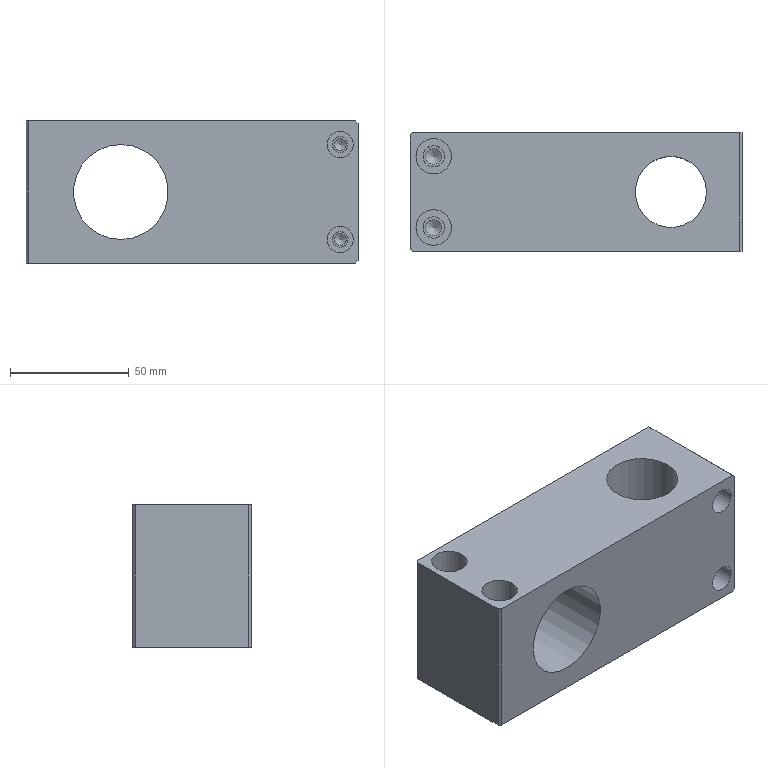Part | NX | 1 solid | 36 faces | box 140 x 50 x 60 mm | volume 301515 mm3 | plane 18 | cylinder 14 | cone 4 | commonest cylinder face diameters 5 x2 6.6 x2 6.8 x2 9 x2 11 x2 15 x2
STEP:
#1=CARTESIAN_POINT('',(62.5,1.5,7.5));
#2=VERTEX_POINT('',#1);
#3=CARTESIAN_POINT('',(62.5,1.5,10.));
#4=DIRECTION('',(0.,-1.,0.));
#5=DIRECTION('',(0.,0.,-1.));
#6=AXIS2_PLACEMENT_3D('',#3,#4,#5);
#7=CIRCLE('',#6,2.5);
#8=EDGE_CURVE('',#2,#2,#7,.T.);
#9=ORIENTED_EDGE('',*,*,#8,.F.);
#10=EDGE_LOOP('',(#9));
#11=FACE_BOUND('',#10,.T.);
#12=CARTESIAN_POINT('',(59.2,1.5,10.));
#13=VERTEX_POINT('',#12);
#14=CARTESIAN_POINT('',(62.5,1.5,10.));
#15=DIRECTION('',(0.,1.,0.));
#16=DIRECTION('',(-1.,0.,0.));
#17=AXIS2_PLACEMENT_3D('',#14,#15,#16);
#18=CIRCLE('',#17,3.3);
#19=EDGE_CURVE('',#13,#13,#18,.T.);
#20=ORIENTED_EDGE('',*,*,#19,.F.);
#21=EDGE_LOOP('',(#20));
#22=FACE_BOUND('',#21,.T.);
#23=CARTESIAN_POINT('',(20.,1.5,60.));
#24=DIRECTION('',(0.,1.,0.));
#25=DIRECTION('',(-1.,0.,0.));
#26=AXIS2_PLACEMENT_3D('',#23,#24,#25);
#27=PLANE('',#26);
#28=ADVANCED_FACE('',(#11,#22),#27,.F.);
#29=CARTESIAN_POINT('',(62.5,1.5,47.5));
#30=VERTEX_POINT('',#29);
#31=CARTESIAN_POINT('',(62.5,1.5,50.));
#32=DIRECTION('',(0.,-1.,0.));
#33=DIRECTION('',(0.,0.,-1.));
#34=AXIS2_PLACEMENT_3D('',#31,#32,#33);
#35=CIRCLE('',#34,2.5);
#36=EDGE_CURVE('',#30,#30,#35,.T.);
#37=ORIENTED_EDGE('',*,*,#36,.F.);
#38=EDGE_LOOP('',(#37));
#39=FACE_BOUND('',#38,.T.);
#40=CARTESIAN_POINT('',(59.2,1.5,50.));
#41=VERTEX_POINT('',#40);
#42=CARTESIAN_POINT('',(62.5,1.5,50.));
#43=DIRECTION('',(0.,1.,0.));
#44=DIRECTION('',(-1.,0.,0.));
#45=AXIS2_PLACEMENT_3D('',#42,#43,#44);
#46=CIRCLE('',#45,3.3);
#47=EDGE_CURVE('',#41,#41,#46,.T.);
#48=ORIENTED_EDGE('',*,*,#47,.F.);
#49=EDGE_LOOP('',(#48));
#50=FACE_BOUND('',#49,.T.);
#51=CARTESIAN_POINT('',(20.,1.5,60.));
#52=DIRECTION('',(0.,1.,0.));
#53=DIRECTION('',(-1.,0.,0.));
#54=AXIS2_PLACEMENT_3D('',#51,#52,#53);
#55=PLANE('',#54);
#56=ADVANCED_FACE('',(#39,#50),#55,.F.);
#57=CARTESIAN_POINT('',(-56.6,-15.,28.5));
#58=VERTEX_POINT('',#57);
#59=CARTESIAN_POINT('',(-60.,-15.,28.5));
#60=DIRECTION('',(0.,0.,1.));
#61=DIRECTION('',(1.,0.,0.));
#62=AXIS2_PLACEMENT_3D('',#59,#60,#61);
#63=CIRCLE('',#62,3.4);
#64=EDGE_CURVE('',#58,#58,#63,.T.);
#65=ORIENTED_EDGE('',*,*,#64,.F.);
#66=EDGE_LOOP('',(#65));
#67=FACE_BOUND('',#66,.T.);
#68=CARTESIAN_POINT('',(-64.5,-15.,28.5));
#69=VERTEX_POINT('',#68);
#70=CARTESIAN_POINT('',(-60.,-15.,28.5));
#71=DIRECTION('',(0.,0.,-1.));
#72=DIRECTION('',(-1.,0.,0.));
#73=AXIS2_PLACEMENT_3D('',#70,#71,#72);
#74=CIRCLE('',#73,4.5);
#75=EDGE_CURVE('',#69,#69,#74,.T.);
#76=ORIENTED_EDGE('',*,*,#75,.F.);
#77=EDGE_LOOP('',(#76));
#78=FACE_BOUND('',#77,.T.);
#79=CARTESIAN_POINT('',(-70.,25.,28.5));
#80=DIRECTION('',(0.,0.,-1.));
#81=DIRECTION('',(-1.,0.,0.));
#82=AXIS2_PLACEMENT_3D('',#79,#80,#81);
#83=PLANE('',#82);
#84=ADVANCED_FACE('',(#67,#78),#83,.F.);
#85=CARTESIAN_POINT('',(-56.6,15.,28.5));
#86=VERTEX_POINT('',#85);
#87=CARTESIAN_POINT('',(-60.,15.,28.5));
#88=DIRECTION('',(0.,0.,1.));
#89=DIRECTION('',(1.,0.,0.));
#90=AXIS2_PLACEMENT_3D('',#87,#88,#89);
#91=CIRCLE('',#90,3.4);
#92=EDGE_CURVE('',#86,#86,#91,.T.);
#93=ORIENTED_EDGE('',*,*,#92,.F.);
#94=EDGE_LOOP('',(#93));
#95=FACE_BOUND('',#94,.T.);
#96=CARTESIAN_POINT('',(-64.5,15.,28.5));
#97=VERTEX_POINT('',#96);
#98=CARTESIAN_POINT('',(-60.,15.,28.5));
#99=DIRECTION('',(0.,0.,-1.));
#100=DIRECTION('',(-1.,0.,0.));
#101=AXIS2_PLACEMENT_3D('',#98,#99,#100);
#102=CIRCLE('',#101,4.5);
#103=EDGE_CURVE('',#97,#97,#102,.T.);
#104=ORIENTED_EDGE('',*,*,#103,.F.);
#105=EDGE_LOOP('',(#104));
#106=FACE_BOUND('',#105,.T.);
#107=CARTESIAN_POINT('',(-70.,25.,28.5));
#108=DIRECTION('',(0.,0.,-1.));
#109=DIRECTION('',(-1.,0.,0.));
#110=AXIS2_PLACEMENT_3D('',#107,#108,#109);
#111=PLANE('',#110);
#112=ADVANCED_FACE('',(#95,#106),#111,.F.);
#113=CARTESIAN_POINT('',(-70.,24.,0.));
#114=VERTEX_POINT('',#113);
#115=CARTESIAN_POINT('',(-69.,25.,0.));
#116=VERTEX_POINT('',#115);
#117=CARTESIAN_POINT('',(-47.,47.,0.));
#118=DIRECTION('',(0.7071,0.7071,0.));
#119=VECTOR('',#118,1000.);
#120=LINE('',#117,#119);
#121=EDGE_CURVE('',#114,#116,#120,.T.);
#122=ORIENTED_EDGE('',*,*,#121,.F.);
#123=CARTESIAN_POINT('',(-70.,24.,60.));
#124=VERTEX_POINT('',#123);
#125=CARTESIAN_POINT('',(-70.,24.,60.));
#126=DIRECTION('',(0.,0.,-1.));
#127=VECTOR('',#126,1000.);
#128=LINE('',#125,#127);
#129=EDGE_CURVE('',#124,#114,#128,.T.);
#130=ORIENTED_EDGE('',*,*,#129,.F.);
#131=CARTESIAN_POINT('',(-69.,25.,60.));
#132=VERTEX_POINT('',#131);
#133=CARTESIAN_POINT('',(-70.,24.,60.));
#134=DIRECTION('',(-0.7071,-0.7071,0.));
#135=VECTOR('',#134,1000.);
#136=LINE('',#133,#135);
#137=EDGE_CURVE('',#132,#124,#136,.T.);
#138=ORIENTED_EDGE('',*,*,#137,.F.);
#139=CARTESIAN_POINT('',(-69.,25.,60.));
#140=DIRECTION('',(0.,0.,1.));
#141=VECTOR('',#140,1000.);
#142=LINE('',#139,#141);
#143=EDGE_CURVE('',#116,#132,#142,.T.);
#144=ORIENTED_EDGE('',*,*,#143,.F.);
#145=EDGE_LOOP('',(#122,#130,#138,#144));
#146=FACE_BOUND('',#145,.T.);
#147=CARTESIAN_POINT('',(-70.,24.,60.));
#148=DIRECTION('',(0.7071,-0.7071,0.));
#149=DIRECTION('',(0.,0.,-1.));
#150=AXIS2_PLACEMENT_3D('',#147,#148,#149);
#151=PLANE('',#150);
#152=ADVANCED_FACE('',(#146),#151,.F.);
#153=CARTESIAN_POINT('',(-69.,-25.,0.));
#154=VERTEX_POINT('',#153);
#155=CARTESIAN_POINT('',(-70.,-24.,0.));
#156=VERTEX_POINT('',#155);
#157=CARTESIAN_POINT('',(-47.,-47.,0.));
#158=DIRECTION('',(-0.7071,0.7071,0.));
#159=VECTOR('',#158,1000.);
#160=LINE('',#157,#159);
#161=EDGE_CURVE('',#154,#156,#160,.T.);
#162=ORIENTED_EDGE('',*,*,#161,.F.);
#163=CARTESIAN_POINT('',(-69.,-25.,60.));
#164=VERTEX_POINT('',#163);
#165=CARTESIAN_POINT('',(-69.,-25.,60.));
#166=DIRECTION('',(0.,0.,-1.));
#167=VECTOR('',#166,1000.);
#168=LINE('',#165,#167);
#169=EDGE_CURVE('',#164,#154,#168,.T.);
#170=ORIENTED_EDGE('',*,*,#169,.F.);
#171=CARTESIAN_POINT('',(-70.,-24.,60.));
#172=VERTEX_POINT('',#171);
#173=CARTESIAN_POINT('',(-69.,-25.,60.));
#174=DIRECTION('',(0.7071,-0.7071,0.));
#175=VECTOR('',#174,1000.);
#176=LINE('',#173,#175);
#177=EDGE_CURVE('',#172,#164,#176,.T.);
#178=ORIENTED_EDGE('',*,*,#177,.F.);
#179=CARTESIAN_POINT('',(-70.,-24.,60.));
#180=DIRECTION('',(0.,0.,1.));
#181=VECTOR('',#180,1000.);
#182=LINE('',#179,#181);
#183=EDGE_CURVE('',#156,#172,#182,.T.);
#184=ORIENTED_EDGE('',*,*,#183,.F.);
#185=EDGE_LOOP('',(#162,#170,#178,#184));
#186=FACE_BOUND('',#185,.T.);
#187=CARTESIAN_POINT('',(-69.,-25.,60.));
#188=DIRECTION('',(0.7071,0.7071,0.));
#189=DIRECTION('',(0.,0.,-1.));
#190=AXIS2_PLACEMENT_3D('',#187,#188,#189);
#191=PLANE('',#190);
#192=ADVANCED_FACE('',(#186),#191,.F.);
#193=CARTESIAN_POINT('',(69.,-25.,60.));
#194=VERTEX_POINT('',#193);
#195=CARTESIAN_POINT('',(69.,25.,60.));
#196=VERTEX_POINT('',#195);
#197=CARTESIAN_POINT('',(69.,0.,60.));
#198=DIRECTION('',(0.,1.,0.));
#199=VECTOR('',#198,1000.);
#200=LINE('',#197,#199);
#201=EDGE_CURVE('',#194,#196,#200,.T.);
#202=ORIENTED_EDGE('',*,*,#201,.F.);
#203=CARTESIAN_POINT('',(70.,-25.,59.));
#204=VERTEX_POINT('',#203);
#205=CARTESIAN_POINT('',(69.,-25.,60.));
#206=DIRECTION('',(-0.7071,0.,0.7071));
#207=VECTOR('',#206,1000.);
#208=LINE('',#205,#207);
#209=EDGE_CURVE('',#204,#194,#208,.T.);
#210=ORIENTED_EDGE('',*,*,#209,.F.);
#211=CARTESIAN_POINT('',(70.,25.,59.));
#212=VERTEX_POINT('',#211);
#213=CARTESIAN_POINT('',(70.,-25.,59.));
#214=DIRECTION('',(0.,-1.,0.));
#215=VECTOR('',#214,1000.);
#216=LINE('',#213,#215);
#217=EDGE_CURVE('',#212,#204,#216,.T.);
#218=ORIENTED_EDGE('',*,*,#217,.F.);
#219=CARTESIAN_POINT('',(69.,25.,60.));
#220=DIRECTION('',(0.7071,0.,-0.7071));
#221=VECTOR('',#220,1000.);
#222=LINE('',#219,#221);
#223=EDGE_CURVE('',#196,#212,#222,.T.);
#224=ORIENTED_EDGE('',*,*,#223,.F.);
#225=EDGE_LOOP('',(#202,#210,#218,#224));
#226=FACE_BOUND('',#225,.T.);
#227=CARTESIAN_POINT('',(69.,0.,60.));
#228=DIRECTION('',(-0.7071,0.,-0.7071));
#229=DIRECTION('',(0.,1.,0.));
#230=AXIS2_PLACEMENT_3D('',#227,#228,#229);
#231=PLANE('',#230);
#232=ADVANCED_FACE('',(#226),#231,.F.);
#233=CARTESIAN_POINT('',(69.,-25.,0.));
#234=VERTEX_POINT('',#233);
#235=CARTESIAN_POINT('',(70.,-25.,1.));
#236=VERTEX_POINT('',#235);
#237=CARTESIAN_POINT('',(70.,-25.,1.));
#238=DIRECTION('',(0.7071,0.,0.7071));
#239=VECTOR('',#238,1000.);
#240=LINE('',#237,#239);
#241=EDGE_CURVE('',#234,#236,#240,.T.);
#242=ORIENTED_EDGE('',*,*,#241,.F.);
#243=CARTESIAN_POINT('',(69.,25.,0.));
#244=VERTEX_POINT('',#243);
#245=CARTESIAN_POINT('',(69.,-25.,0.));
#246=DIRECTION('',(0.,-1.,0.));
#247=VECTOR('',#246,1000.);
#248=LINE('',#245,#247);
#249=EDGE_CURVE('',#244,#234,#248,.T.);
#250=ORIENTED_EDGE('',*,*,#249,.F.);
#251=CARTESIAN_POINT('',(70.,25.,1.));
#252=VERTEX_POINT('',#251);
#253=CARTESIAN_POINT('',(70.,25.,1.));
#254=DIRECTION('',(-0.7071,0.,-0.7071));
#255=VECTOR('',#254,1000.);
#256=LINE('',#253,#255);
#257=EDGE_CURVE('',#252,#244,#256,.T.);
#258=ORIENTED_EDGE('',*,*,#257,.F.);
#259=CARTESIAN_POINT('',(70.,-1.5,1.));
#260=DIRECTION('',(0.,1.,0.));
#261=VECTOR('',#260,1000.);
#262=LINE('',#259,#261);
#263=EDGE_CURVE('',#236,#252,#262,.T.);
#264=ORIENTED_EDGE('',*,*,#263,.F.);
#265=EDGE_LOOP('',(#242,#250,#258,#264));
#266=FACE_BOUND('',#265,.T.);
#267=CARTESIAN_POINT('',(70.,-25.,1.));
#268=DIRECTION('',(0.7071,0.,-0.7071));
#269=DIRECTION('',(0.,-1.,0.));
#270=AXIS2_PLACEMENT_3D('',#267,#268,#269);
#271=PLANE('',#270);
#272=ADVANCED_FACE('',(#266),#271,.T.);
#273=CARTESIAN_POINT('',(-52.5,15.,45.));
#274=VERTEX_POINT('',#273);
#275=CARTESIAN_POINT('',(-60.,15.,45.));
#276=DIRECTION('',(0.,0.,1.));
#277=DIRECTION('',(1.,0.,0.));
#278=AXIS2_PLACEMENT_3D('',#275,#276,#277);
#279=CIRCLE('',#278,7.5);
#280=EDGE_CURVE('',#274,#274,#279,.T.);
#281=ORIENTED_EDGE('',*,*,#280,.T.);
#282=EDGE_LOOP('',(#281));
#283=FACE_BOUND('',#282,.T.);
#284=CARTESIAN_POINT('',(-55.5,15.,45.));
#285=VERTEX_POINT('',#284);
#286=CARTESIAN_POINT('',(-60.,15.,45.));
#287=DIRECTION('',(0.,0.,1.));
#288=DIRECTION('',(1.,0.,0.));
#289=AXIS2_PLACEMENT_3D('',#286,#287,#288);
#290=CIRCLE('',#289,4.5);
#291=EDGE_CURVE('',#285,#285,#290,.T.);
#292=ORIENTED_EDGE('',*,*,#291,.F.);
#293=EDGE_LOOP('',(#292));
#294=FACE_BOUND('',#293,.T.);
#295=CARTESIAN_POINT('',(-55.5,15.,45.));
#296=DIRECTION('',(0.,0.,-1.));
#297=DIRECTION('',(-1.,0.,0.));
#298=AXIS2_PLACEMENT_3D('',#295,#296,#297);
#299=PLANE('',#298);
#300=ADVANCED_FACE('',(#283,#294),#299,.F.);
#301=CARTESIAN_POINT('',(-67.5,-15.,45.));
#302=VERTEX_POINT('',#301);
#303=CARTESIAN_POINT('',(-60.,-15.,45.));
#304=DIRECTION('',(0.,0.,1.));
#305=DIRECTION('',(-1.,0.,0.));
#306=AXIS2_PLACEMENT_3D('',#303,#304,#305);
#307=CIRCLE('',#306,7.5);
#308=EDGE_CURVE('',#302,#302,#307,.T.);
#309=ORIENTED_EDGE('',*,*,#308,.T.);
#310=EDGE_LOOP('',(#309));
#311=FACE_BOUND('',#310,.T.);
#312=CARTESIAN_POINT('',(-64.5,-15.,45.));
#313=VERTEX_POINT('',#312);
#314=CARTESIAN_POINT('',(-60.,-15.,45.));
#315=DIRECTION('',(0.,0.,1.));
#316=DIRECTION('',(-1.,0.,0.));
#317=AXIS2_PLACEMENT_3D('',#314,#315,#316);
#318=CIRCLE('',#317,4.5);
#319=EDGE_CURVE('',#313,#313,#318,.T.);
#320=ORIENTED_EDGE('',*,*,#319,.F.);
#321=EDGE_LOOP('',(#320));
#322=FACE_BOUND('',#321,.T.);
#323=CARTESIAN_POINT('',(-55.5,15.,45.));
#324=DIRECTION('',(0.,0.,-1.));
#325=DIRECTION('',(-1.,0.,0.));
#326=AXIS2_PLACEMENT_3D('',#323,#324,#325);
#327=PLANE('',#326);
#328=ADVANCED_FACE('',(#311,#322),#327,.F.);
#329=CARTESIAN_POINT('',(62.5,-10.,44.5));
#330=VERTEX_POINT('',#329);
#331=CARTESIAN_POINT('',(62.5,-10.,50.));
#332=DIRECTION('',(0.,-1.,0.));
#333=DIRECTION('',(0.,0.,-1.));
#334=AXIS2_PLACEMENT_3D('',#331,#332,#333);
#335=CIRCLE('',#334,5.5);
#336=EDGE_CURVE('',#330,#330,#335,.T.);
#337=ORIENTED_EDGE('',*,*,#336,.T.);
#338=EDGE_LOOP('',(#337));
#339=FACE_BOUND('',#338,.T.);
#340=CARTESIAN_POINT('',(62.5,-10.,46.7));
#341=VERTEX_POINT('',#340);
#342=CARTESIAN_POINT('',(62.5,-10.,50.));
#343=DIRECTION('',(0.,-1.,0.));
#344=DIRECTION('',(0.,0.,-1.));
#345=AXIS2_PLACEMENT_3D('',#342,#343,#344);
#346=CIRCLE('',#345,3.3);
#347=EDGE_CURVE('',#341,#341,#346,.T.);
#348=ORIENTED_EDGE('',*,*,#347,.F.);
#349=EDGE_LOOP('',(#348));
#350=FACE_BOUND('',#349,.T.);
#351=CARTESIAN_POINT('',(65.8,-10.,50.));
#352=DIRECTION('',(0.,1.,0.));
#353=DIRECTION('',(0.,0.,1.));
#354=AXIS2_PLACEMENT_3D('',#351,#352,#353);
#355=PLANE('',#354);
#356=ADVANCED_FACE('',(#339,#350),#355,.F.);
#357=CARTESIAN_POINT('',(62.5,-10.,15.5));
#358=VERTEX_POINT('',#357);
#359=CARTESIAN_POINT('',(62.5,-10.,10.));
#360=DIRECTION('',(0.,-1.,0.));
#361=DIRECTION('',(0.,0.,1.));
#362=AXIS2_PLACEMENT_3D('',#359,#360,#361);
#363=CIRCLE('',#362,5.5);
#364=EDGE_CURVE('',#358,#358,#363,.T.);
#365=ORIENTED_EDGE('',*,*,#364,.T.);
#366=EDGE_LOOP('',(#365));
#367=FACE_BOUND('',#366,.T.);
#368=CARTESIAN_POINT('',(62.5,-10.,13.3));
#369=VERTEX_POINT('',#368);
#370=CARTESIAN_POINT('',(62.5,-10.,10.));
#371=DIRECTION('',(0.,-1.,0.));
#372=DIRECTION('',(0.,0.,1.));
#373=AXIS2_PLACEMENT_3D('',#370,#371,#372);
#374=CIRCLE('',#373,3.3);
#375=EDGE_CURVE('',#369,#369,#374,.T.);
#376=ORIENTED_EDGE('',*,*,#375,.F.);
#377=EDGE_LOOP('',(#376));
#378=FACE_BOUND('',#377,.T.);
#379=CARTESIAN_POINT('',(65.8,-10.,50.));
#380=DIRECTION('',(0.,1.,0.));
#381=DIRECTION('',(0.,0.,1.));
#382=AXIS2_PLACEMENT_3D('',#379,#380,#381);
#383=PLANE('',#382);
#384=ADVANCED_FACE('',(#367,#378),#383,.F.);
#385=CARTESIAN_POINT('',(-70.,25.,0.));
#386=DIRECTION('',(-1.,0.,0.));
#387=VECTOR('',#386,1000.);
#388=LINE('',#385,#387);
#389=EDGE_CURVE('',#244,#116,#388,.T.);
#390=ORIENTED_EDGE('',*,*,#389,.F.);
#391=ORIENTED_EDGE('',*,*,#249,.T.);
#392=CARTESIAN_POINT('',(-70.,-25.,0.));
#393=DIRECTION('',(1.,0.,0.));
#394=VECTOR('',#393,1000.);
#395=LINE('',#392,#394);
#396=EDGE_CURVE('',#154,#234,#395,.T.);
#397=ORIENTED_EDGE('',*,*,#396,.F.);
#398=ORIENTED_EDGE('',*,*,#161,.T.);
#399=CARTESIAN_POINT('',(-70.,-25.,0.));
#400=DIRECTION('',(0.,-1.,0.));
#401=VECTOR('',#400,1000.);
#402=LINE('',#399,#401);
#403=EDGE_CURVE('',#114,#156,#402,.T.);
#404=ORIENTED_EDGE('',*,*,#403,.F.);
#405=ORIENTED_EDGE('',*,*,#121,.T.);
#406=EDGE_LOOP('',(#390,#391,#397,#398,#404,#405));
#407=FACE_BOUND('',#406,.T.);
#408=CARTESIAN_POINT('',(55.,0.,0.));
#409=VERTEX_POINT('',#408);
#410=CARTESIAN_POINT('',(40.,0.,0.));
#411=DIRECTION('',(0.,0.,1.));
#412=DIRECTION('',(1.,0.,0.));
#413=AXIS2_PLACEMENT_3D('',#410,#411,#412);
#414=CIRCLE('',#413,15.);
#415=EDGE_CURVE('',#409,#409,#414,.T.);
#416=ORIENTED_EDGE('',*,*,#415,.T.);
#417=EDGE_LOOP('',(#416));
#418=FACE_BOUND('',#417,.T.);
#419=CARTESIAN_POINT('',(0.,0.,0.));
#420=DIRECTION('',(0.,0.,-1.));
#421=DIRECTION('',(-1.,0.,0.));
#422=AXIS2_PLACEMENT_3D('',#419,#420,#421);
#423=PLANE('',#422);
#424=ADVANCED_FACE('',(#407,#418),#423,.T.);
#425=CARTESIAN_POINT('',(-30.,-25.,50.));
#426=VERTEX_POINT('',#425);
#427=CARTESIAN_POINT('',(-30.,-25.,30.));
#428=DIRECTION('',(0.,1.,0.));
#429=DIRECTION('',(0.,0.,1.));
#430=AXIS2_PLACEMENT_3D('',#427,#428,#429);
#431=CIRCLE('',#430,20.);
#432=EDGE_CURVE('',#426,#426,#431,.T.);
#433=ORIENTED_EDGE('',*,*,#432,.T.);
#434=EDGE_LOOP('',(#433));
#435=FACE_BOUND('',#434,.T.);
#436=ORIENTED_EDGE('',*,*,#396,.T.);
#437=ORIENTED_EDGE('',*,*,#241,.T.);
#438=CARTESIAN_POINT('',(70.,-25.,60.));
#439=DIRECTION('',(0.,0.,-1.));
#440=VECTOR('',#439,1000.);
#441=LINE('',#438,#440);
#442=EDGE_CURVE('',#204,#236,#441,.T.);
#443=ORIENTED_EDGE('',*,*,#442,.F.);
#444=ORIENTED_EDGE('',*,*,#209,.T.);
#445=CARTESIAN_POINT('',(-70.,-25.,60.));
#446=DIRECTION('',(1.,0.,0.));
#447=VECTOR('',#446,1000.);
#448=LINE('',#445,#447);
#449=EDGE_CURVE('',#164,#194,#448,.T.);
#450=ORIENTED_EDGE('',*,*,#449,.F.);
#451=ORIENTED_EDGE('',*,*,#169,.T.);
#452=EDGE_LOOP('',(#436,#437,#443,#444,#450,#451));
#453=FACE_BOUND('',#452,.T.);
#454=CARTESIAN_POINT('',(62.5,-25.,4.5));
#455=VERTEX_POINT('',#454);
#456=CARTESIAN_POINT('',(62.5,-25.,10.));
#457=DIRECTION('',(0.,-1.,0.));
#458=DIRECTION('',(0.,0.,-1.));
#459=AXIS2_PLACEMENT_3D('',#456,#457,#458);
#460=CIRCLE('',#459,5.5);
#461=EDGE_CURVE('',#455,#455,#460,.T.);
#462=ORIENTED_EDGE('',*,*,#461,.F.);
#463=EDGE_LOOP('',(#462));
#464=FACE_BOUND('',#463,.T.);
#465=CARTESIAN_POINT('',(62.5,-25.,44.5));
#466=VERTEX_POINT('',#465);
#467=CARTESIAN_POINT('',(62.5,-25.,50.));
#468=DIRECTION('',(0.,-1.,0.));
#469=DIRECTION('',(0.,0.,-1.));
#470=AXIS2_PLACEMENT_3D('',#467,#468,#469);
#471=CIRCLE('',#470,5.5);
#472=EDGE_CURVE('',#466,#466,#471,.T.);
#473=ORIENTED_EDGE('',*,*,#472,.F.);
#474=EDGE_LOOP('',(#473));
#475=FACE_BOUND('',#474,.T.);
#476=CARTESIAN_POINT('',(-70.,-25.,60.));
#477=DIRECTION('',(0.,1.,0.));
#478=DIRECTION('',(0.,0.,1.));
#479=AXIS2_PLACEMENT_3D('',#476,#477,#478);
#480=PLANE('',#479);
#481=ADVANCED_FACE('',(#435,#453,#464,#475),#480,.F.);
#482=CARTESIAN_POINT('',(-30.,25.,50.));
#483=VERTEX_POINT('',#482);
#484=CARTESIAN_POINT('',(-30.,25.,30.));
#485=DIRECTION('',(0.,1.,0.));
#486=DIRECTION('',(0.,0.,1.));
#487=AXIS2_PLACEMENT_3D('',#484,#485,#486);
#488=CIRCLE('',#487,20.);
#489=EDGE_CURVE('',#483,#483,#488,.T.);
#490=ORIENTED_EDGE('',*,*,#489,.F.);
#491=EDGE_LOOP('',(#490));
#492=FACE_BOUND('',#491,.T.);
#493=CARTESIAN_POINT('',(70.,25.,60.));
#494=DIRECTION('',(0.,0.,-1.));
#495=VECTOR('',#494,1000.);
#496=LINE('',#493,#495);
#497=EDGE_CURVE('',#212,#252,#496,.T.);
#498=ORIENTED_EDGE('',*,*,#497,.T.);
#499=ORIENTED_EDGE('',*,*,#257,.T.);
#500=ORIENTED_EDGE('',*,*,#389,.T.);
#501=ORIENTED_EDGE('',*,*,#143,.T.);
#502=CARTESIAN_POINT('',(-70.,25.,60.));
#503=DIRECTION('',(-1.,0.,0.));
#504=VECTOR('',#503,1000.);
#505=LINE('',#502,#504);
#506=EDGE_CURVE('',#196,#132,#505,.T.);
#507=ORIENTED_EDGE('',*,*,#506,.F.);
#508=ORIENTED_EDGE('',*,*,#223,.T.);
#509=EDGE_LOOP('',(#498,#499,#500,#501,#507,#508));
#510=FACE_BOUND('',#509,.T.);
#511=CARTESIAN_POINT('',(-70.,25.,60.));
#512=DIRECTION('',(0.,-1.,0.));
#513=DIRECTION('',(0.,0.,-1.));
#514=AXIS2_PLACEMENT_3D('',#511,#512,#513);
#515=PLANE('',#514);
#516=ADVANCED_FACE('',(#492,#510),#515,.F.);
#517=CARTESIAN_POINT('',(-70.,-25.,60.));
#518=DIRECTION('',(0.,-1.,0.));
#519=VECTOR('',#518,1000.);
#520=LINE('',#517,#519);
#521=EDGE_CURVE('',#124,#172,#520,.T.);
#522=ORIENTED_EDGE('',*,*,#521,.F.);
#523=ORIENTED_EDGE('',*,*,#129,.T.);
#524=ORIENTED_EDGE('',*,*,#403,.T.);
#525=ORIENTED_EDGE('',*,*,#183,.T.);
#526=EDGE_LOOP('',(#522,#523,#524,#525));
#527=FACE_BOUND('',#526,.T.);
#528=CARTESIAN_POINT('',(-70.,-25.,60.));
#529=DIRECTION('',(1.,0.,0.));
#530=DIRECTION('',(0.,0.,-1.));
#531=AXIS2_PLACEMENT_3D('',#528,#529,#530);
#532=PLANE('',#531);
#533=ADVANCED_FACE('',(#527),#532,.F.);
#534=ORIENTED_EDGE('',*,*,#415,.F.);
#535=EDGE_LOOP('',(#534));
#536=FACE_BOUND('',#535,.T.);
#537=CARTESIAN_POINT('',(55.,0.,60.));
#538=VERTEX_POINT('',#537);
#539=CARTESIAN_POINT('',(40.,0.,60.));
#540=DIRECTION('',(0.,0.,1.));
#541=DIRECTION('',(1.,0.,0.));
#542=AXIS2_PLACEMENT_3D('',#539,#540,#541);
#543=CIRCLE('',#542,15.);
#544=EDGE_CURVE('',#538,#538,#543,.T.);
#545=ORIENTED_EDGE('',*,*,#544,.T.);
#546=EDGE_LOOP('',(#545));
#547=FACE_BOUND('',#546,.T.);
#548=CARTESIAN_POINT('',(40.,0.,0.));
#549=DIRECTION('',(0.,0.,1.));
#550=DIRECTION('',(1.,0.,0.));
#551=AXIS2_PLACEMENT_3D('',#548,#549,#550);
#552=CYLINDRICAL_SURFACE('',#551,15.);
#553=ADVANCED_FACE('',(#536,#547),#552,.F.);
#554=ORIENTED_EDGE('',*,*,#442,.T.);
#555=ORIENTED_EDGE('',*,*,#263,.T.);
#556=ORIENTED_EDGE('',*,*,#497,.F.);
#557=ORIENTED_EDGE('',*,*,#217,.T.);
#558=EDGE_LOOP('',(#554,#555,#556,#557));
#559=FACE_BOUND('',#558,.T.);
#560=CARTESIAN_POINT('',(70.,-25.,60.));
#561=DIRECTION('',(-1.,0.,0.));
#562=DIRECTION('',(0.,0.,1.));
#563=AXIS2_PLACEMENT_3D('',#560,#561,#562);
#564=PLANE('',#563);
#565=ADVANCED_FACE('',(#559),#564,.F.);
#566=ORIENTED_EDGE('',*,*,#449,.T.);
#567=ORIENTED_EDGE('',*,*,#201,.T.);
#568=ORIENTED_EDGE('',*,*,#506,.T.);
#569=ORIENTED_EDGE('',*,*,#137,.T.);
#570=ORIENTED_EDGE('',*,*,#521,.T.);
#571=ORIENTED_EDGE('',*,*,#177,.T.);
#572=EDGE_LOOP('',(#566,#567,#568,#569,#570,#571));
#573=FACE_BOUND('',#572,.T.);
#574=CARTESIAN_POINT('',(-52.5,15.,60.));
#575=VERTEX_POINT('',#574);
#576=CARTESIAN_POINT('',(-60.,15.,60.));
#577=DIRECTION('',(0.,0.,1.));
#578=DIRECTION('',(1.,0.,0.));
#579=AXIS2_PLACEMENT_3D('',#576,#577,#578);
#580=CIRCLE('',#579,7.5);
#581=EDGE_CURVE('',#575,#575,#580,.T.);
#582=ORIENTED_EDGE('',*,*,#581,.F.);
#583=EDGE_LOOP('',(#582));
#584=FACE_BOUND('',#583,.T.);
#585=ORIENTED_EDGE('',*,*,#544,.F.);
#586=EDGE_LOOP('',(#585));
#587=FACE_BOUND('',#586,.T.);
#588=CARTESIAN_POINT('',(-52.5,-15.,60.));
#589=VERTEX_POINT('',#588);
#590=CARTESIAN_POINT('',(-60.,-15.,60.));
#591=DIRECTION('',(0.,0.,1.));
#592=DIRECTION('',(1.,0.,0.));
#593=AXIS2_PLACEMENT_3D('',#590,#591,#592);
#594=CIRCLE('',#593,7.5);
#595=EDGE_CURVE('',#589,#589,#594,.T.);
#596=ORIENTED_EDGE('',*,*,#595,.F.);
#597=EDGE_LOOP('',(#596));
#598=FACE_BOUND('',#597,.T.);
#599=CARTESIAN_POINT('',(0.,0.,60.));
#600=DIRECTION('',(0.,0.,-1.));
#601=DIRECTION('',(-1.,0.,0.));
#602=AXIS2_PLACEMENT_3D('',#599,#600,#601);
#603=PLANE('',#602);
#604=ADVANCED_FACE('',(#573,#584,#587,#598),#603,.F.);
#605=ORIENTED_EDGE('',*,*,#489,.T.);
#606=EDGE_LOOP('',(#605));
#607=FACE_BOUND('',#606,.T.);
#608=ORIENTED_EDGE('',*,*,#432,.F.);
#609=EDGE_LOOP('',(#608));
#610=FACE_BOUND('',#609,.T.);
#611=CARTESIAN_POINT('',(-30.,-25.,30.));
#612=DIRECTION('',(0.,1.,0.));
#613=DIRECTION('',(0.,0.,1.));
#614=AXIS2_PLACEMENT_3D('',#611,#612,#613);
#615=CYLINDRICAL_SURFACE('',#614,20.);
#616=ADVANCED_FACE('',(#607,#610),#615,.F.);
#617=ORIENTED_EDGE('',*,*,#375,.T.);
#618=EDGE_LOOP('',(#617));
#619=FACE_BOUND('',#618,.T.);
#620=ORIENTED_EDGE('',*,*,#19,.T.);
#621=EDGE_LOOP('',(#620));
#622=FACE_BOUND('',#621,.T.);
#623=CARTESIAN_POINT('',(62.5,-25.,10.));
#624=DIRECTION('',(0.,-1.,0.));
#625=DIRECTION('',(0.,0.,-1.));
#626=AXIS2_PLACEMENT_3D('',#623,#624,#625);
#627=CYLINDRICAL_SURFACE('',#626,3.3);
#628=ADVANCED_FACE('',(#619,#622),#627,.F.);
#629=ORIENTED_EDGE('',*,*,#461,.T.);
#630=EDGE_LOOP('',(#629));
#631=FACE_BOUND('',#630,.T.);
#632=ORIENTED_EDGE('',*,*,#364,.F.);
#633=EDGE_LOOP('',(#632));
#634=FACE_BOUND('',#633,.T.);
#635=CARTESIAN_POINT('',(62.5,-25.,10.));
#636=DIRECTION('',(0.,-1.,0.));
#637=DIRECTION('',(0.,0.,-1.));
#638=AXIS2_PLACEMENT_3D('',#635,#636,#637);
#639=CYLINDRICAL_SURFACE('',#638,5.5);
#640=ADVANCED_FACE('',(#631,#634),#639,.F.);
#641=ORIENTED_EDGE('',*,*,#347,.T.);
#642=EDGE_LOOP('',(#641));
#643=FACE_BOUND('',#642,.T.);
#644=ORIENTED_EDGE('',*,*,#47,.T.);
#645=EDGE_LOOP('',(#644));
#646=FACE_BOUND('',#645,.T.);
#647=CARTESIAN_POINT('',(62.5,-25.,50.));
#648=DIRECTION('',(0.,-1.,0.));
#649=DIRECTION('',(0.,0.,-1.));
#650=AXIS2_PLACEMENT_3D('',#647,#648,#649);
#651=CYLINDRICAL_SURFACE('',#650,3.3);
#652=ADVANCED_FACE('',(#643,#646),#651,.F.);
#653=ORIENTED_EDGE('',*,*,#472,.T.);
#654=EDGE_LOOP('',(#653));
#655=FACE_BOUND('',#654,.T.);
#656=ORIENTED_EDGE('',*,*,#336,.F.);
#657=EDGE_LOOP('',(#656));
#658=FACE_BOUND('',#657,.T.);
#659=CARTESIAN_POINT('',(62.5,-25.,50.));
#660=DIRECTION('',(0.,-1.,0.));
#661=DIRECTION('',(0.,0.,-1.));
#662=AXIS2_PLACEMENT_3D('',#659,#660,#661);
#663=CYLINDRICAL_SURFACE('',#662,5.5);
#664=ADVANCED_FACE('',(#655,#658),#663,.F.);
#665=ORIENTED_EDGE('',*,*,#75,.T.);
#666=EDGE_LOOP('',(#665));
#667=FACE_BOUND('',#666,.T.);
#668=ORIENTED_EDGE('',*,*,#319,.T.);
#669=EDGE_LOOP('',(#668));
#670=FACE_BOUND('',#669,.T.);
#671=CARTESIAN_POINT('',(-60.,-15.,60.));
#672=DIRECTION('',(0.,0.,1.));
#673=DIRECTION('',(1.,0.,0.));
#674=AXIS2_PLACEMENT_3D('',#671,#672,#673);
#675=CYLINDRICAL_SURFACE('',#674,4.5);
#676=ADVANCED_FACE('',(#667,#670),#675,.F.);
#677=ORIENTED_EDGE('',*,*,#308,.F.);
#678=EDGE_LOOP('',(#677));
#679=FACE_BOUND('',#678,.T.);
#680=ORIENTED_EDGE('',*,*,#595,.T.);
#681=EDGE_LOOP('',(#680));
#682=FACE_BOUND('',#681,.T.);
#683=CARTESIAN_POINT('',(-60.,-15.,60.));
#684=DIRECTION('',(0.,0.,1.));
#685=DIRECTION('',(1.,0.,0.));
#686=AXIS2_PLACEMENT_3D('',#683,#684,#685);
#687=CYLINDRICAL_SURFACE('',#686,7.5);
#688=ADVANCED_FACE('',(#679,#682),#687,.F.);
#689=ORIENTED_EDGE('',*,*,#103,.T.);
#690=EDGE_LOOP('',(#689));
#691=FACE_BOUND('',#690,.T.);
#692=ORIENTED_EDGE('',*,*,#291,.T.);
#693=EDGE_LOOP('',(#692));
#694=FACE_BOUND('',#693,.T.);
#695=CARTESIAN_POINT('',(-60.,15.,60.));
#696=DIRECTION('',(0.,0.,1.));
#697=DIRECTION('',(1.,0.,0.));
#698=AXIS2_PLACEMENT_3D('',#695,#696,#697);
#699=CYLINDRICAL_SURFACE('',#698,4.5);
#700=ADVANCED_FACE('',(#691,#694),#699,.F.);
#701=ORIENTED_EDGE('',*,*,#280,.F.);
#702=EDGE_LOOP('',(#701));
#703=FACE_BOUND('',#702,.T.);
#704=ORIENTED_EDGE('',*,*,#581,.T.);
#705=EDGE_LOOP('',(#704));
#706=FACE_BOUND('',#705,.T.);
#707=CARTESIAN_POINT('',(-60.,15.,60.));
#708=DIRECTION('',(0.,0.,1.));
#709=DIRECTION('',(1.,0.,0.));
#710=AXIS2_PLACEMENT_3D('',#707,#708,#709);
#711=CYLINDRICAL_SURFACE('',#710,7.5);
#712=ADVANCED_FACE('',(#703,#706),#711,.F.);
#713=CARTESIAN_POINT('',(62.5,18.002,10.));
#714=VERTEX_POINT('',#713);
#715=VERTEX_LOOP('',#714);
#716=FACE_BOUND('',#715,.T.);
#717=CARTESIAN_POINT('',(62.5,16.5,7.5));
#718=VERTEX_POINT('',#717);
#719=CARTESIAN_POINT('',(62.5,16.5,10.));
#720=DIRECTION('',(0.,-1.,0.));
#721=DIRECTION('',(0.,0.,-1.));
#722=AXIS2_PLACEMENT_3D('',#719,#720,#721);
#723=CIRCLE('',#722,2.5);
#724=EDGE_CURVE('',#718,#718,#723,.T.);
#725=ORIENTED_EDGE('',*,*,#724,.T.);
#726=EDGE_LOOP('',(#725));
#727=FACE_BOUND('',#726,.T.);
#728=CARTESIAN_POINT('',(62.5,16.5,10.));
#729=DIRECTION('',(0.,-1.,0.));
#730=DIRECTION('',(0.,0.,-1.));
#731=AXIS2_PLACEMENT_3D('',#728,#729,#730);
#732=CONICAL_SURFACE('',#731,2.5,1.03);
#733=ADVANCED_FACE('',(#716,#727),#732,.F.);
#734=ORIENTED_EDGE('',*,*,#8,.T.);
#735=EDGE_LOOP('',(#734));
#736=FACE_BOUND('',#735,.T.);
#737=ORIENTED_EDGE('',*,*,#724,.F.);
#738=EDGE_LOOP('',(#737));
#739=FACE_BOUND('',#738,.T.);
#740=CARTESIAN_POINT('',(62.5,1.5,10.));
#741=DIRECTION('',(0.,-1.,0.));
#742=DIRECTION('',(0.,0.,-1.));
#743=AXIS2_PLACEMENT_3D('',#740,#741,#742);
#744=CYLINDRICAL_SURFACE('',#743,2.5);
#745=ADVANCED_FACE('',(#736,#739),#744,.F.);
#746=CARTESIAN_POINT('',(62.5,18.002,50.));
#747=VERTEX_POINT('',#746);
#748=VERTEX_LOOP('',#747);
#749=FACE_BOUND('',#748,.T.);
#750=CARTESIAN_POINT('',(62.5,16.5,47.5));
#751=VERTEX_POINT('',#750);
#752=CARTESIAN_POINT('',(62.5,16.5,50.));
#753=DIRECTION('',(0.,-1.,0.));
#754=DIRECTION('',(0.,0.,-1.));
#755=AXIS2_PLACEMENT_3D('',#752,#753,#754);
#756=CIRCLE('',#755,2.5);
#757=EDGE_CURVE('',#751,#751,#756,.T.);
#758=ORIENTED_EDGE('',*,*,#757,.T.);
#759=EDGE_LOOP('',(#758));
#760=FACE_BOUND('',#759,.T.);
#761=CARTESIAN_POINT('',(62.5,16.5,50.));
#762=DIRECTION('',(0.,-1.,0.));
#763=DIRECTION('',(0.,0.,-1.));
#764=AXIS2_PLACEMENT_3D('',#761,#762,#763);
#765=CONICAL_SURFACE('',#764,2.5,1.03);
#766=ADVANCED_FACE('',(#749,#760),#765,.F.);
#767=ORIENTED_EDGE('',*,*,#36,.T.);
#768=EDGE_LOOP('',(#767));
#769=FACE_BOUND('',#768,.T.);
#770=ORIENTED_EDGE('',*,*,#757,.F.);
#771=EDGE_LOOP('',(#770));
#772=FACE_BOUND('',#771,.T.);
#773=CARTESIAN_POINT('',(62.5,1.5,50.));
#774=DIRECTION('',(0.,-1.,0.));
#775=DIRECTION('',(0.,0.,-1.));
#776=AXIS2_PLACEMENT_3D('',#773,#774,#775);
#777=CYLINDRICAL_SURFACE('',#776,2.5);
#778=ADVANCED_FACE('',(#769,#772),#777,.F.);
#779=CARTESIAN_POINT('',(-56.6,-15.,8.75));
#780=VERTEX_POINT('',#779);
#781=CARTESIAN_POINT('',(-60.,-15.,8.75));
#782=DIRECTION('',(0.,0.,1.));
#783=DIRECTION('',(1.,0.,0.));
#784=AXIS2_PLACEMENT_3D('',#781,#782,#783);
#785=CIRCLE('',#784,3.4);
#786=EDGE_CURVE('',#780,#780,#785,.T.);
#787=ORIENTED_EDGE('',*,*,#786,.T.);
#788=EDGE_LOOP('',(#787));
#789=FACE_BOUND('',#788,.T.);
#790=CARTESIAN_POINT('',(-60.,-15.,6.707));
#791=VERTEX_POINT('',#790);
#792=VERTEX_LOOP('',#791);
#793=FACE_BOUND('',#792,.T.);
#794=CARTESIAN_POINT('',(-60.,-15.,8.75));
#795=DIRECTION('',(0.,0.,1.));
#796=DIRECTION('',(1.,0.,0.));
#797=AXIS2_PLACEMENT_3D('',#794,#795,#796);
#798=CONICAL_SURFACE('',#797,3.4,1.03);
#799=ADVANCED_FACE('',(#789,#793),#798,.F.);
#800=ORIENTED_EDGE('',*,*,#786,.F.);
#801=EDGE_LOOP('',(#800));
#802=FACE_BOUND('',#801,.T.);
#803=ORIENTED_EDGE('',*,*,#64,.T.);
#804=EDGE_LOOP('',(#803));
#805=FACE_BOUND('',#804,.T.);
#806=CARTESIAN_POINT('',(-60.,-15.,28.5));
#807=DIRECTION('',(0.,0.,1.));
#808=DIRECTION('',(1.,0.,0.));
#809=AXIS2_PLACEMENT_3D('',#806,#807,#808);
#810=CYLINDRICAL_SURFACE('',#809,3.4);
#811=ADVANCED_FACE('',(#802,#805),#810,.F.);
#812=CARTESIAN_POINT('',(-56.6,15.,8.75));
#813=VERTEX_POINT('',#812);
#814=CARTESIAN_POINT('',(-60.,15.,8.75));
#815=DIRECTION('',(0.,0.,1.));
#816=DIRECTION('',(1.,0.,0.));
#817=AXIS2_PLACEMENT_3D('',#814,#815,#816);
#818=CIRCLE('',#817,3.4);
#819=EDGE_CURVE('',#813,#813,#818,.T.);
#820=ORIENTED_EDGE('',*,*,#819,.T.);
#821=EDGE_LOOP('',(#820));
#822=FACE_BOUND('',#821,.T.);
#823=CARTESIAN_POINT('',(-60.,15.,6.707));
#824=VERTEX_POINT('',#823);
#825=VERTEX_LOOP('',#824);
#826=FACE_BOUND('',#825,.T.);
#827=CARTESIAN_POINT('',(-60.,15.,8.75));
#828=DIRECTION('',(0.,0.,1.));
#829=DIRECTION('',(1.,0.,0.));
#830=AXIS2_PLACEMENT_3D('',#827,#828,#829);
#831=CONICAL_SURFACE('',#830,3.4,1.03);
#832=ADVANCED_FACE('',(#822,#826),#831,.F.);
#833=ORIENTED_EDGE('',*,*,#819,.F.);
#834=EDGE_LOOP('',(#833));
#835=FACE_BOUND('',#834,.T.);
#836=ORIENTED_EDGE('',*,*,#92,.T.);
#837=EDGE_LOOP('',(#836));
#838=FACE_BOUND('',#837,.T.);
#839=CARTESIAN_POINT('',(-60.,15.,28.5));
#840=DIRECTION('',(0.,0.,1.));
#841=DIRECTION('',(1.,0.,0.));
#842=AXIS2_PLACEMENT_3D('',#839,#840,#841);
#843=CYLINDRICAL_SURFACE('',#842,3.4);
#844=ADVANCED_FACE('',(#835,#838),#843,.F.);
#845=CLOSED_SHELL('',(#28,#56,#84,#112,#152,#192,#232,#272,#300,#328,#356,#384,#424,#481,#516,#533,#553,#565,#604,#616,#628,#640,#652,#664,#676,#688,#700,#712,#733,#745,#766,#778,#799,#811,#832,#844));
#846=MANIFOLD_SOLID_BREP('',#845);
#847=(LENGTH_UNIT()NAMED_UNIT(*)SI_UNIT(.MILLI.,.METRE.));
#848=UNCERTAINTY_MEASURE_WITH_UNIT(LENGTH_MEASURE(0.00001),#847,'','');
#849=(NAMED_UNIT(*)PLANE_ANGLE_UNIT()SI_UNIT($,.RADIAN.));
#850=(NAMED_UNIT(*)SI_UNIT($,.STERADIAN.)SOLID_ANGLE_UNIT());
#851=(GEOMETRIC_REPRESENTATION_CONTEXT(3)GLOBAL_UNCERTAINTY_ASSIGNED_CONTEXT((#848))GLOBAL_UNIT_ASSIGNED_CONTEXT((#847,#849,#850))REPRESENTATION_CONTEXT('',''));
#852=ADVANCED_BREP_SHAPE_REPRESENTATION('',(#846),#851);